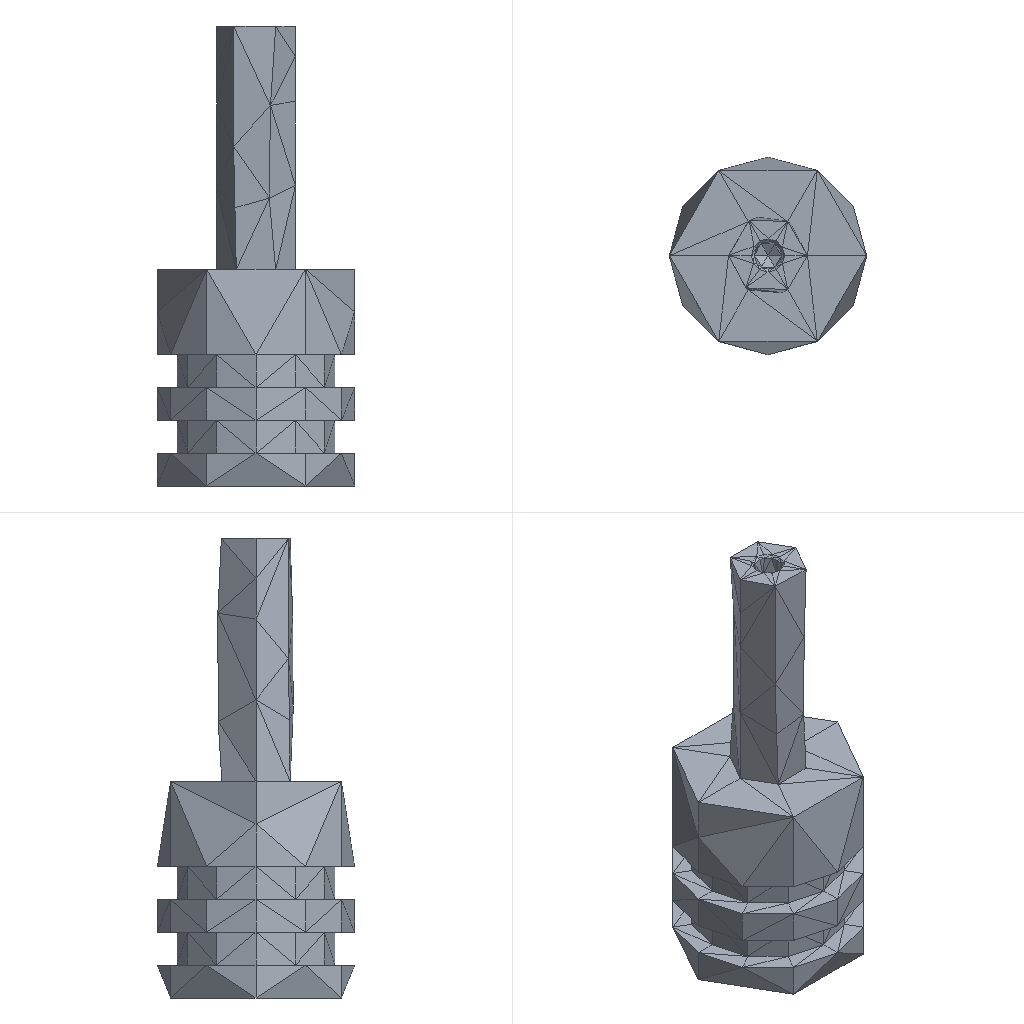Simulation study | ansys workbench
Ansys APDL input file, long lists of numbers shortened:
/batch
/config,noeldb,1     ! force off writing results to database
*get,_wallstrt,active,,time,wall
! ANSYS input file written by Workbench version 2022 R1
! File used for geometry attach: F:\ansys（分析文件汇总)\ansys刀片有限元分析\装配体\轴.STEP
/title,2222--____ (G5)
! ****** Begin Custom Load Command Snippet ******
/COM, ACT Extensions:
/COM,     LSDYNA, 2021.1
/COM,
! ****** End   Custom Load Command Snippet ******
*DIM,_wb_ProjectScratch_dir,string,248
_wb_ProjectScratch_dir(1) = 'F:\ansys（分析文件汇总)\ansys刀片有限元分析\_ProjectScratch\Scr5BEB\'
*DIM,_wb_SolverFiles_dir,string,248
_wb_SolverFiles_dir(1) = 'F:\ansys（分析文件汇总)\ansys刀片有限元分析\2222_files\dp0\SYS-4\MECH\'
*DIM,_wb_userfiles_dir,string,248
_wb_userfiles_dir(1) = 'F:\ansys（分析文件汇总)\ansys刀片有限元分析\2222_files\user_files\'
/com,--- Data in consistent NMM units. See Solving Units in the help system for more information.
/units,MPA
/nopr
/wb,file,start              !  signify a WB generated input file
/prep7
! Turn off shape checking because checks already performed inside WB mesher.
! See help system for more information.
SHPP,OFF,,NOWARN
/nolist
etcon,set             ! allow ANSYS to choose best KEYOP's for 180x elements, resets any applicable keyopt to MAPDL defaults
/com,*********** Nodes for the whole assembly ***********
nblock,3,,1324
(1i9,3e20.9e3)
        1     1.500000000E+01     1.836970199E-15     3.300000000E+01
! (1203 more lines like these left out)
-1
/com,*********** Nodes for all Remote Points ***********
nblock,3
(1i9,3e20.9e3)
     1205     1.856511411E-16     0.000000000E+00     3.780905181E+01
-1
/wb,elem,start            !  set before creation of elements
/com,*********** Elements for Body 1 "_-FreeParts|____(____)1" ***********
et,1,187
eblock,19,solid,,591
(19i9)
        1        1        1        1        0        0        0        0       10        0        1       69      210      166      205      699     1126      694      697
! (1181 more lines like these left out)
-1
/wb,elem,end               !  done creating elements
/com,*********** Send User Defined Coordinate System(s) ***********
csys,0
toffst,273.15,  ! Temperature offset from absolute zero
/com,*********** Set Reference Temperature ***********
tref,22.
/wb,mat,start              !  starting to send materials
/com,*********** Send Materials ***********
Temperature = 'TEMP' ! Temperature
MP,DENS,1,7.85e-09,	! tonne mm^-3
MP,ALPX,1,1.2e-05,	! C^-1
MP,C,1,434000000,	! mm^2 s^-2 C^-1
MP,KXX,1,60.5,	! tonne mm s^-3 C^-1
MP,RSVX,1,0.00017,	! ohm mm
MP,EX,1,200000,	! tonne s^-2 mm^-1
MP,NUXY,1,0.3,
MP,MURX,1,10000,
/wb,mat,end                !  done sending materials
!************************* Model Summary ********************
!_-FreeParts|____(____)1,	结构钢,	matid,	1
!************************* End Model Summary ********************
! get the diagonal of the bounding box. Needed later for other things
*get,_xmin,node,,mnloc,x
*get,_ymin,node,,mnloc,y
*get,_zmin,node,,mnloc,z
*get,_xmax,node,,mxloc,x
*get,_ymax,node,,mxloc,y
*get,_zmax,node,,mxloc,z
_ASMDIAG=(_xmax-_xmin)*(_xmax-_xmin)+(_ymax-_ymin)*(_ymax-_ymin)+(_zmax-_zmin)*(_zmax-_zmin)
_ASMDIAG=SQRT(_ASMDIAG)
/wb,contact,start          !  starting to send contact
/wb,contact,end            !  done creating contacts
/golist
/wb,load,start             !  starting to send loads
/com,*********** Fixed Supports ***********
CMBLOCK,_FIXEDSU,NODE,      182
(8i10)
        29        30        31        32        37        38        39        40
! (22 more lines like these left out)
cmsel,s,_FIXEDSU
d,all,all
nsel,all
/com,*********** Create Remote Point "内部远程点" ***********
! -------- Remote Point Used by "力矩" --------
*set,tid,3
*set,cid,2
et,cid,174
et,tid,170
keyo,tid,2,1               ! Don't fix the pilot node
keyo,tid,4,111111
keyo,cid,12,5              ! Bonded Contact
keyo,cid,4,1               ! Deformable RBE3 style load
keyo,cid,2,2               ! MPC style contact
eblock,10,,,74
(15i9)
      981        2        2        2        0       18       17      186      186      307      313      186      321
! (73 more lines like these left out)
-1
*set,_npilot,1205
_npilot33=_npilot
type,tid
mat ,cid
real,cid
tshape,pilo
en,1055,_npilot
tshape
/com,*********** Construct Moment Using Remote Attachment ***********
/gst,on,on
fini
*get,_numnode,node,0,count
*get,_numelem,elem,0,count
*get, _MAXELEMNUM, elem, 0, NUM, MAX
*get, _MAXNODENUM, node, 0, NUM, MAX
*get, _MAXELEMTYPE, etyp, 0, NUM, MAX
*get, _MAXREALCONST, real, 0, NUM, MAX
/go
/wb,load,end               !  done creating loads
/com,--- Number of total nodes = %_numnode%
/com,--- Number of contact elements = 74
/com,--- Number of spring elements = 0
/com,--- Number of bearing elements = 0
/com,--- Number of solid elements = 591
/com,--- Number of condensed parts = 0
/com,--- Number of total elements = %_numelem%
*get,_wallbsol,active,,time,wall
/com,****************************************************************************
/com,*************************    SOLUTION       ********************************
/com,****************************************************************************
/solu
antype,0                   ! static analysis
_thickRatio=  0     ! Ratio of thick parts in the model
eqsl,sparse,,,,,1
cntr,print,1               ! print out contact info and also make no initial contact an error
dmpoption,emat,no             ! Don't combine emat file for DANSYS
dmpoption,esav,no             ! Don't combine esav file for DANSYS
nldiag,cont,iter           ! print out contact info each equilibrium iteration
rescontrol,,none                 ! Do not keep any restart files
/com,****************************************************
/com,******************* SOLVE FOR LS 1 OF 1 ****************
nsel,s,node,,1205
f,all,mx,0.
f,all,my,0.
f,all,mz,52000.
nsel,all
/nopr
/gopr
nsub,1,1,1
time,1.
outres,erase
outres,all,none
outres,nsol,all,
outres,rsol,all
outres,eangl,all
outres,etmp,all
outres,veng,all
outres,strs,all,
outres,epel,all,
outres,eppl,all,
outres,cont,all,
! *********** WB SOLVE COMMAND ***********
! check interactive state
*get,ANSINTER_,active,,int
*if,ANSINTER_,ne,0,then
/eof
*endif
solve
/com *************** Write FE CONNECTORS *********
CEWRITE,file,ce,,INTE
/com,****************************************************
/com,*************** FINISHED SOLVE FOR LS 1 *************
*get,_wallasol,active,,time,wall
/nopr
*get,_numnode,node,0,count
*get,_numelem,elem,0,count
*get, _MAXELEMNUM, elem, 0, NUM, MAX
*get, _MAXNODENUM, node, 0, NUM, MAX,,,INTERNAL
*get, _MAXELEMTYPE, etyp, 0, NUM, MAX
*get, _MAXREALCONST, real, 0, NUM, MAX
/gopr
/post1
xmlo,ENCODING,ISO-8859-1
xmlo,parm
/xml,parm,xml
fini
/gopr
*get,_walldone,active,,time,wall
_preptime=(_wallbsol-_wallstrt)*3600
_solvtime=(_wallasol-_wallbsol)*3600
_posttime=(_walldone-_wallasol)*3600
_totaltim=(_walldone-_wallstrt)*3600
*get,_dlbratio,active,0,solu,dlbr
*get,_combtime,active,0,solu,comb
*get,_ssmode,active,0,solu,ssmm
*get,_ndofs,active,0,solu,ndof
*get,_sol_end_time,active,0,set,time
*if,_sol_end_time,eq,1.,then
/fclean				!clean distributed files
*endif
/com,--- Total number of nodes = %_numnode%
/com,--- Total number of elements = %_numelem%
/com,--- Element load balance ratio = %_dlbratio%
/com,--- Time to combine distributed files = %_combtime%
/com,--- Sparse memory mode = %_ssmode%
/com,--- Number of DOF = %_ndofs%
/wb,file,end               ! done with WB generated input